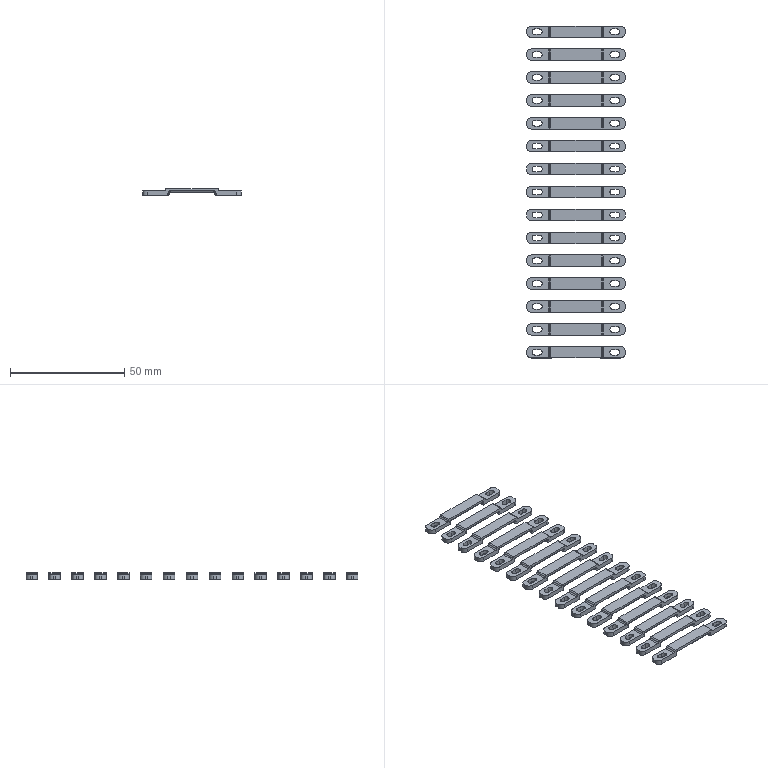Part | 15 solids | 660 faces | box 43 x 145 x 3 mm | volume 5226 mm3 | cylinder 360 | plane 240 | torus 60 | commonest cylinder face diameters 1 x210 2.4 x90 4 x60